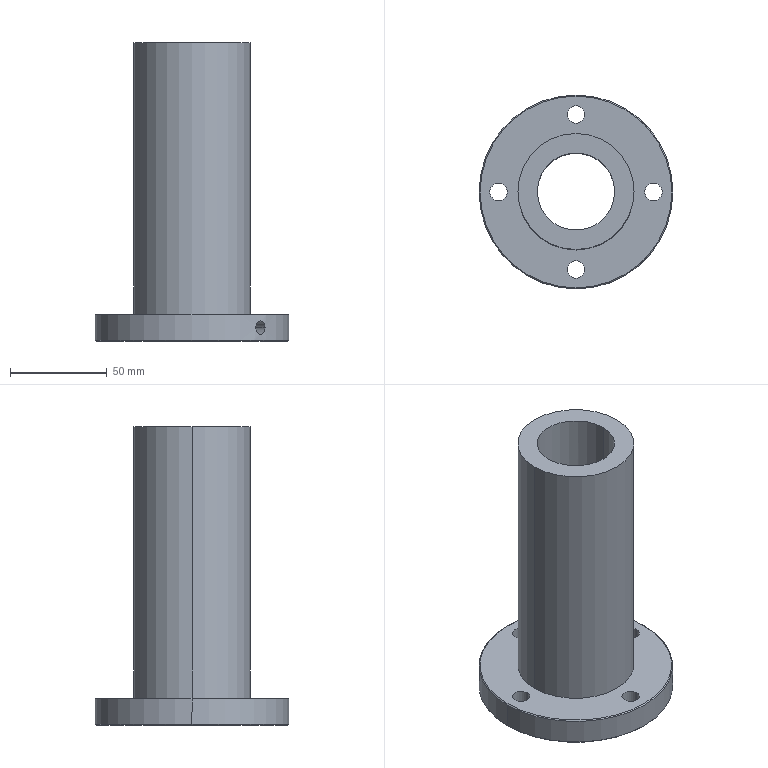Part | SolidWorks | features BaseBody 1 | 1 solid | 25 faces | box 100 x 100 x 154 mm | volume 306400 mm3 | cylinder 18 | cone 4 | plane 3 | commonest cylinder face diameters 9 x8 6.88 x4 40 x2 60 x2 100 x2
STEP:
#1=CARTESIAN_POINT('',(-30.,0.,147.));
#2=VERTEX_POINT('',#1);
#3=CARTESIAN_POINT('',(30.,0.,147.));
#4=VERTEX_POINT('',#3);
#5=CARTESIAN_POINT('',(0.,0.,147.));
#6=DIRECTION('',(0.,0.,-1.));
#7=DIRECTION('',(-1.,0.,0.));
#8=AXIS2_PLACEMENT_3D('',#5,#6,#7);
#9=CIRCLE('',#8,30.);
#10=EDGE_CURVE('',#2,#4,#9,.T.);
#11=ORIENTED_EDGE('',*,*,#10,.T.);
#12=CARTESIAN_POINT('',(30.,0.,7.));
#13=VERTEX_POINT('',#12);
#14=CARTESIAN_POINT('',(30.,0.,147.));
#15=DIRECTION('',(0.,0.,-1.));
#16=VECTOR('',#15,1000.);
#17=LINE('',#14,#16);
#18=EDGE_CURVE('',#4,#13,#17,.T.);
#19=ORIENTED_EDGE('',*,*,#18,.T.);
#20=CARTESIAN_POINT('',(-30.,0.,7.));
#21=VERTEX_POINT('',#20);
#22=CARTESIAN_POINT('',(0.,0.,7.));
#23=DIRECTION('',(0.,0.,1.));
#24=DIRECTION('',(-1.,0.,0.));
#25=AXIS2_PLACEMENT_3D('',#22,#23,#24);
#26=CIRCLE('',#25,30.);
#27=EDGE_CURVE('',#13,#21,#26,.T.);
#28=ORIENTED_EDGE('',*,*,#27,.T.);
#29=CARTESIAN_POINT('',(-30.,0.,147.));
#30=DIRECTION('',(0.,0.,-1.));
#31=VECTOR('',#30,1000.);
#32=LINE('',#29,#31);
#33=EDGE_CURVE('',#2,#21,#32,.T.);
#34=ORIENTED_EDGE('',*,*,#33,.F.);
#35=EDGE_LOOP('',(#11,#19,#28,#34));
#36=FACE_OUTER_BOUND('',#35,.T.);
#37=CARTESIAN_POINT('',(0.,0.,147.));
#38=DIRECTION('',(0.,0.,-1.));
#39=DIRECTION('',(-1.,0.,0.));
#40=AXIS2_PLACEMENT_3D('',#37,#38,#39);
#41=CYLINDRICAL_SURFACE('',#40,30.);
#42=ADVANCED_FACE('',(#36),#41,.T.);
#43=CARTESIAN_POINT('',(-4.5,-40.,-7.));
#44=VERTEX_POINT('',#43);
#45=CARTESIAN_POINT('',(4.5,-40.,-7.));
#46=VERTEX_POINT('',#45);
#47=CARTESIAN_POINT('',(0.,-40.,-7.));
#48=DIRECTION('',(0.,0.,1.));
#49=DIRECTION('',(1.,0.,0.));
#50=AXIS2_PLACEMENT_3D('',#47,#48,#49);
#51=CIRCLE('',#50,4.5);
#52=EDGE_CURVE('',#44,#46,#51,.T.);
#53=ORIENTED_EDGE('',*,*,#52,.F.);
#54=CARTESIAN_POINT('',(-4.5,-40.,7.));
#55=VERTEX_POINT('',#54);
#56=CARTESIAN_POINT('',(-4.5,-40.,-7.));
#57=DIRECTION('',(0.,0.,1.));
#58=VECTOR('',#57,1000.);
#59=LINE('',#56,#58);
#60=EDGE_CURVE('',#44,#55,#59,.T.);
#61=ORIENTED_EDGE('',*,*,#60,.T.);
#62=CARTESIAN_POINT('',(4.5,-40.,7.));
#63=VERTEX_POINT('',#62);
#64=CARTESIAN_POINT('',(0.,-40.,7.));
#65=DIRECTION('',(0.,0.,-1.));
#66=DIRECTION('',(1.,0.,0.));
#67=AXIS2_PLACEMENT_3D('',#64,#65,#66);
#68=CIRCLE('',#67,4.5);
#69=EDGE_CURVE('',#63,#55,#68,.T.);
#70=ORIENTED_EDGE('',*,*,#69,.F.);
#71=CARTESIAN_POINT('',(4.5,-40.,-7.));
#72=DIRECTION('',(0.,0.,1.));
#73=VECTOR('',#72,1000.);
#74=LINE('',#71,#73);
#75=EDGE_CURVE('',#46,#63,#74,.T.);
#76=ORIENTED_EDGE('',*,*,#75,.F.);
#77=EDGE_LOOP('',(#53,#61,#70,#76));
#78=FACE_OUTER_BOUND('',#77,.T.);
#79=CARTESIAN_POINT('',(0.,-40.,-7.));
#80=DIRECTION('',(0.,0.,1.));
#81=DIRECTION('',(1.,0.,0.));
#82=AXIS2_PLACEMENT_3D('',#79,#80,#81);
#83=CYLINDRICAL_SURFACE('',#82,4.5);
#84=ADVANCED_FACE('',(#78),#83,.F.);
#85=CARTESIAN_POINT('',(35.5,0.,-7.));
#86=VERTEX_POINT('',#85);
#87=CARTESIAN_POINT('',(44.5,0.,-7.));
#88=VERTEX_POINT('',#87);
#89=CARTESIAN_POINT('',(40.,0.,-7.));
#90=DIRECTION('',(0.,0.,1.));
#91=DIRECTION('',(1.,0.,0.));
#92=AXIS2_PLACEMENT_3D('',#89,#90,#91);
#93=CIRCLE('',#92,4.5);
#94=EDGE_CURVE('',#86,#88,#93,.T.);
#95=ORIENTED_EDGE('',*,*,#94,.F.);
#96=CARTESIAN_POINT('',(35.5,0.,7.));
#97=VERTEX_POINT('',#96);
#98=CARTESIAN_POINT('',(35.5,0.,-7.));
#99=DIRECTION('',(0.,0.,1.));
#100=VECTOR('',#99,1000.);
#101=LINE('',#98,#100);
#102=EDGE_CURVE('',#86,#97,#101,.T.);
#103=ORIENTED_EDGE('',*,*,#102,.T.);
#104=CARTESIAN_POINT('',(44.5,0.,7.));
#105=VERTEX_POINT('',#104);
#106=CARTESIAN_POINT('',(40.,0.,7.));
#107=DIRECTION('',(0.,0.,-1.));
#108=DIRECTION('',(1.,0.,0.));
#109=AXIS2_PLACEMENT_3D('',#106,#107,#108);
#110=CIRCLE('',#109,4.5);
#111=EDGE_CURVE('',#105,#97,#110,.T.);
#112=ORIENTED_EDGE('',*,*,#111,.F.);
#113=CARTESIAN_POINT('',(44.5,0.,-7.));
#114=DIRECTION('',(0.,0.,1.));
#115=VECTOR('',#114,1000.);
#116=LINE('',#113,#115);
#117=EDGE_CURVE('',#88,#105,#116,.T.);
#118=ORIENTED_EDGE('',*,*,#117,.F.);
#119=EDGE_LOOP('',(#95,#103,#112,#118));
#120=FACE_OUTER_BOUND('',#119,.T.);
#121=CARTESIAN_POINT('',(40.,0.,-7.));
#122=DIRECTION('',(0.,0.,1.));
#123=DIRECTION('',(1.,0.,0.));
#124=AXIS2_PLACEMENT_3D('',#121,#122,#123);
#125=CYLINDRICAL_SURFACE('',#124,4.5);
#126=ADVANCED_FACE('',(#120),#125,.F.);
#127=CARTESIAN_POINT('',(-4.5,40.,-7.));
#128=VERTEX_POINT('',#127);
#129=CARTESIAN_POINT('',(4.5,40.,-7.));
#130=VERTEX_POINT('',#129);
#131=CARTESIAN_POINT('',(0.,40.,-7.));
#132=DIRECTION('',(0.,0.,1.));
#133=DIRECTION('',(1.,0.,0.));
#134=AXIS2_PLACEMENT_3D('',#131,#132,#133);
#135=CIRCLE('',#134,4.5);
#136=EDGE_CURVE('',#128,#130,#135,.T.);
#137=ORIENTED_EDGE('',*,*,#136,.F.);
#138=CARTESIAN_POINT('',(-4.5,40.,7.));
#139=VERTEX_POINT('',#138);
#140=CARTESIAN_POINT('',(-4.5,40.,-7.));
#141=DIRECTION('',(0.,0.,1.));
#142=VECTOR('',#141,1000.);
#143=LINE('',#140,#142);
#144=EDGE_CURVE('',#128,#139,#143,.T.);
#145=ORIENTED_EDGE('',*,*,#144,.T.);
#146=CARTESIAN_POINT('',(4.5,40.,7.));
#147=VERTEX_POINT('',#146);
#148=CARTESIAN_POINT('',(0.,40.,7.));
#149=DIRECTION('',(0.,0.,-1.));
#150=DIRECTION('',(1.,0.,0.));
#151=AXIS2_PLACEMENT_3D('',#148,#149,#150);
#152=CIRCLE('',#151,4.5);
#153=EDGE_CURVE('',#147,#139,#152,.T.);
#154=ORIENTED_EDGE('',*,*,#153,.F.);
#155=CARTESIAN_POINT('',(4.5,40.,-7.));
#156=DIRECTION('',(0.,0.,1.));
#157=VECTOR('',#156,1000.);
#158=LINE('',#155,#157);
#159=EDGE_CURVE('',#130,#147,#158,.T.);
#160=ORIENTED_EDGE('',*,*,#159,.F.);
#161=EDGE_LOOP('',(#137,#145,#154,#160));
#162=FACE_OUTER_BOUND('',#161,.T.);
#163=CARTESIAN_POINT('',(0.,40.,-7.));
#164=DIRECTION('',(0.,0.,1.));
#165=DIRECTION('',(1.,0.,0.));
#166=AXIS2_PLACEMENT_3D('',#163,#164,#165);
#167=CYLINDRICAL_SURFACE('',#166,4.5);
#168=ADVANCED_FACE('',(#162),#167,.F.);
#169=CARTESIAN_POINT('',(-44.5,0.,-7.));
#170=VERTEX_POINT('',#169);
#171=CARTESIAN_POINT('',(-35.5,0.,-7.));
#172=VERTEX_POINT('',#171);
#173=CARTESIAN_POINT('',(-40.,0.,-7.));
#174=DIRECTION('',(0.,0.,1.));
#175=DIRECTION('',(1.,0.,0.));
#176=AXIS2_PLACEMENT_3D('',#173,#174,#175);
#177=CIRCLE('',#176,4.5);
#178=EDGE_CURVE('',#170,#172,#177,.T.);
#179=ORIENTED_EDGE('',*,*,#178,.F.);
#180=CARTESIAN_POINT('',(-44.5,0.,7.));
#181=VERTEX_POINT('',#180);
#182=CARTESIAN_POINT('',(-44.5,0.,-7.));
#183=DIRECTION('',(0.,0.,1.));
#184=VECTOR('',#183,1000.);
#185=LINE('',#182,#184);
#186=EDGE_CURVE('',#170,#181,#185,.T.);
#187=ORIENTED_EDGE('',*,*,#186,.T.);
#188=CARTESIAN_POINT('',(-35.5,0.,7.));
#189=VERTEX_POINT('',#188);
#190=CARTESIAN_POINT('',(-40.,0.,7.));
#191=DIRECTION('',(0.,0.,-1.));
#192=DIRECTION('',(1.,0.,0.));
#193=AXIS2_PLACEMENT_3D('',#190,#191,#192);
#194=CIRCLE('',#193,4.5);
#195=EDGE_CURVE('',#189,#181,#194,.T.);
#196=ORIENTED_EDGE('',*,*,#195,.F.);
#197=CARTESIAN_POINT('',(-35.5,0.,-7.));
#198=DIRECTION('',(0.,0.,1.));
#199=VECTOR('',#198,1000.);
#200=LINE('',#197,#199);
#201=EDGE_CURVE('',#172,#189,#200,.T.);
#202=ORIENTED_EDGE('',*,*,#201,.F.);
#203=EDGE_LOOP('',(#179,#187,#196,#202));
#204=FACE_OUTER_BOUND('',#203,.T.);
#205=CARTESIAN_POINT('',(-40.,0.,-7.));
#206=DIRECTION('',(0.,0.,1.));
#207=DIRECTION('',(1.,0.,0.));
#208=AXIS2_PLACEMENT_3D('',#205,#206,#207);
#209=CYLINDRICAL_SURFACE('',#208,4.5);
#210=ADVANCED_FACE('',(#204),#209,.F.);
#211=CARTESIAN_POINT('',(49.5,0.,7.));
#212=VERTEX_POINT('',#211);
#213=CARTESIAN_POINT('',(-49.5,0.,7.));
#214=VERTEX_POINT('',#213);
#215=CARTESIAN_POINT('',(0.,0.,7.));
#216=DIRECTION('',(0.,0.,1.));
#217=DIRECTION('',(-1.,0.,0.));
#218=AXIS2_PLACEMENT_3D('',#215,#216,#217);
#219=CIRCLE('',#218,49.5);
#220=EDGE_CURVE('',#212,#214,#219,.T.);
#221=ORIENTED_EDGE('',*,*,#220,.F.);
#222=CARTESIAN_POINT('',(50.,0.,6.5));
#223=VERTEX_POINT('',#222);
#224=CARTESIAN_POINT('',(50.,0.,6.5));
#225=DIRECTION('',(0.7071,0.,-0.7071));
#226=VECTOR('',#225,1000.);
#227=LINE('',#224,#226);
#228=EDGE_CURVE('',#212,#223,#227,.T.);
#229=ORIENTED_EDGE('',*,*,#228,.T.);
#230=CARTESIAN_POINT('',(-50.,0.,6.5));
#231=VERTEX_POINT('',#230);
#232=CARTESIAN_POINT('',(0.,0.,6.5));
#233=DIRECTION('',(0.,0.,1.));
#234=DIRECTION('',(-1.,0.,0.));
#235=AXIS2_PLACEMENT_3D('',#232,#233,#234);
#236=CIRCLE('',#235,50.);
#237=EDGE_CURVE('',#223,#231,#236,.T.);
#238=ORIENTED_EDGE('',*,*,#237,.T.);
#239=CARTESIAN_POINT('',(-50.,0.,6.5));
#240=DIRECTION('',(-0.7071,0.,-0.7071));
#241=VECTOR('',#240,1000.);
#242=LINE('',#239,#241);
#243=EDGE_CURVE('',#214,#231,#242,.T.);
#244=ORIENTED_EDGE('',*,*,#243,.F.);
#245=EDGE_LOOP('',(#221,#229,#238,#244));
#246=FACE_OUTER_BOUND('',#245,.T.);
#247=CARTESIAN_POINT('',(0.,0.,6.5));
#248=DIRECTION('',(0.,0.,-1.));
#249=DIRECTION('',(-1.,0.,0.));
#250=AXIS2_PLACEMENT_3D('',#247,#248,#249);
#251=CONICAL_SURFACE('',#250,50.,0.7854);
#252=ADVANCED_FACE('',(#246),#251,.T.);
#253=CARTESIAN_POINT('',(11.499,-16.364,0.));
#254=VERTEX_POINT('',#253);
#255=CARTESIAN_POINT('',(16.364,-11.499,0.));
#256=VERTEX_POINT('',#255);
#257=CARTESIAN_POINT('',(11.499,-16.364,0.));
#258=CARTESIAN_POINT('',(11.499,-16.364,0.2277));
#259=CARTESIAN_POINT('',(11.518,-16.351,0.4515));
#260=CARTESIAN_POINT('',(11.59,-16.299,0.8916));
#261=CARTESIAN_POINT('',(11.645,-16.26,1.11));
#262=CARTESIAN_POINT('',(11.787,-16.158,1.527));
#263=CARTESIAN_POINT('',(11.873,-16.095,1.724));
#264=CARTESIAN_POINT('',(12.075,-15.944,2.098));
#265=CARTESIAN_POINT('',(12.192,-15.855,2.274));
#266=CARTESIAN_POINT('',(12.443,-15.659,2.591));
#267=CARTESIAN_POINT('',(12.579,-15.55,2.733));
#268=CARTESIAN_POINT('',(12.87,-15.31,2.985));
#269=CARTESIAN_POINT('',(13.023,-15.181,3.091));
#270=CARTESIAN_POINT('',(13.335,-14.907,3.263));
#271=CARTESIAN_POINT('',(13.496,-14.762,3.329));
#272=CARTESIAN_POINT('',(13.821,-14.458,3.418));
#273=CARTESIAN_POINT('',(13.981,-14.303,3.44));
#274=CARTESIAN_POINT('',(14.299,-13.985,3.44));
#275=CARTESIAN_POINT('',(14.458,-13.821,3.418));
#276=CARTESIAN_POINT('',(14.76,-13.498,3.33));
#277=CARTESIAN_POINT('',(14.904,-13.339,3.265));
#278=CARTESIAN_POINT('',(15.179,-13.024,3.092));
#279=CARTESIAN_POINT('',(15.309,-12.871,2.985));
#280=CARTESIAN_POINT('',(15.547,-12.582,2.736));
#281=CARTESIAN_POINT('',(15.657,-12.445,2.594));
#282=CARTESIAN_POINT('',(15.856,-12.191,2.274));
#283=CARTESIAN_POINT('',(15.942,-12.077,2.101));
#284=CARTESIAN_POINT('',(16.093,-11.875,1.729));
#285=CARTESIAN_POINT('',(16.158,-11.787,1.527));
#286=CARTESIAN_POINT('',(16.26,-11.645,1.112));
#287=CARTESIAN_POINT('',(16.299,-11.591,0.8972));
#288=CARTESIAN_POINT('',(16.35,-11.518,0.4556));
#289=CARTESIAN_POINT('',(16.364,-11.499,0.2277));
#290=CARTESIAN_POINT('',(16.364,-11.499,0.));
#291=B_SPLINE_CURVE_WITH_KNOTS('',3,(#257,#258,#259,#260,#261,#262,#263,#264,#265,#266,#267,#268,#269,#270,#271,#272,#273,#274,#275,#276,#277,#278,#279,#280,#281,#282,#283,#284,#285,#286,#287,#288,#289,#290),.UNSPECIFIED.,.F.,.F.,(4,2,2,2,2,2,2,2,2,2,2,2,2,2,2,2,4),(0.,0.0006733,0.001347,0.00202,0.002693,0.003366,0.00404,0.004713,0.005386,0.006059,0.006733,0.007406,0.008079,0.008753,0.009426,0.0101,0.01077),.UNSPECIFIED.);
#292=EDGE_CURVE('',#254,#256,#291,.T.);
#293=ORIENTED_EDGE('',*,*,#292,.F.);
#294=CARTESIAN_POINT('',(16.364,-11.499,0.));
#295=CARTESIAN_POINT('',(16.364,-11.499,-0.2277));
#296=CARTESIAN_POINT('',(16.351,-11.518,-0.4515));
#297=CARTESIAN_POINT('',(16.299,-11.59,-0.8916));
#298=CARTESIAN_POINT('',(16.26,-11.645,-1.11));
#299=CARTESIAN_POINT('',(16.158,-11.787,-1.527));
#300=CARTESIAN_POINT('',(16.095,-11.873,-1.724));
#301=CARTESIAN_POINT('',(15.944,-12.075,-2.098));
#302=CARTESIAN_POINT('',(15.855,-12.192,-2.274));
#303=CARTESIAN_POINT('',(15.659,-12.443,-2.591));
#304=CARTESIAN_POINT('',(15.55,-12.579,-2.733));
#305=CARTESIAN_POINT('',(15.31,-12.87,-2.985));
#306=CARTESIAN_POINT('',(15.181,-13.023,-3.091));
#307=CARTESIAN_POINT('',(14.907,-13.335,-3.263));
#308=CARTESIAN_POINT('',(14.762,-13.496,-3.329));
#309=CARTESIAN_POINT('',(14.458,-13.821,-3.418));
#310=CARTESIAN_POINT('',(14.303,-13.981,-3.44));
#311=CARTESIAN_POINT('',(13.985,-14.299,-3.44));
#312=CARTESIAN_POINT('',(13.821,-14.458,-3.418));
#313=CARTESIAN_POINT('',(13.498,-14.76,-3.33));
#314=CARTESIAN_POINT('',(13.339,-14.904,-3.265));
#315=CARTESIAN_POINT('',(13.024,-15.179,-3.092));
#316=CARTESIAN_POINT('',(12.871,-15.309,-2.985));
#317=CARTESIAN_POINT('',(12.582,-15.547,-2.736));
#318=CARTESIAN_POINT('',(12.445,-15.657,-2.594));
#319=CARTESIAN_POINT('',(12.191,-15.856,-2.274));
#320=CARTESIAN_POINT('',(12.077,-15.942,-2.101));
#321=CARTESIAN_POINT('',(11.875,-16.093,-1.729));
#322=CARTESIAN_POINT('',(11.787,-16.158,-1.527));
#323=CARTESIAN_POINT('',(11.645,-16.26,-1.112));
#324=CARTESIAN_POINT('',(11.591,-16.299,-0.8972));
#325=CARTESIAN_POINT('',(11.518,-16.35,-0.4556));
#326=CARTESIAN_POINT('',(11.499,-16.364,-0.2277));
#327=CARTESIAN_POINT('',(11.499,-16.364,0.));
#328=B_SPLINE_CURVE_WITH_KNOTS('',3,(#294,#295,#296,#297,#298,#299,#300,#301,#302,#303,#304,#305,#306,#307,#308,#309,#310,#311,#312,#313,#314,#315,#316,#317,#318,#319,#320,#321,#322,#323,#324,#325,#326,#327),.UNSPECIFIED.,.F.,.F.,(4,2,2,2,2,2,2,2,2,2,2,2,2,2,2,2,4),(0.01077,0.01145,0.01212,0.01279,0.01347,0.01414,0.01481,0.01549,0.01616,0.01683,0.01751,0.01818,0.01885,0.01952,0.0202,0.02087,0.02154),.UNSPECIFIED.);
#329=EDGE_CURVE('',#256,#254,#328,.T.);
#330=ORIENTED_EDGE('',*,*,#329,.F.);
#331=EDGE_LOOP('',(#293,#330));
#332=FACE_BOUND('',#331,.T.);
#333=CARTESIAN_POINT('',(20.,0.,147.));
#334=VERTEX_POINT('',#333);
#335=CARTESIAN_POINT('',(-20.,0.,147.));
#336=VERTEX_POINT('',#335);
#337=CARTESIAN_POINT('',(0.,0.,147.));
#338=DIRECTION('',(0.,0.,-1.));
#339=DIRECTION('',(-1.,0.,0.));
#340=AXIS2_PLACEMENT_3D('',#337,#338,#339);
#341=CIRCLE('',#340,20.);
#342=EDGE_CURVE('',#334,#336,#341,.T.);
#343=ORIENTED_EDGE('',*,*,#342,.F.);
#344=CARTESIAN_POINT('',(20.,0.,-7.));
#345=VERTEX_POINT('',#344);
#346=CARTESIAN_POINT('',(20.,0.,7.));
#347=DIRECTION('',(0.,0.,-1.));
#348=VECTOR('',#347,1000.);
#349=LINE('',#346,#348);
#350=EDGE_CURVE('',#334,#345,#349,.T.);
#351=ORIENTED_EDGE('',*,*,#350,.T.);
#352=CARTESIAN_POINT('',(-20.,0.,-7.));
#353=VERTEX_POINT('',#352);
#354=CARTESIAN_POINT('',(0.,0.,-7.));
#355=DIRECTION('',(0.,0.,1.));
#356=DIRECTION('',(-1.,0.,0.));
#357=AXIS2_PLACEMENT_3D('',#354,#355,#356);
#358=CIRCLE('',#357,20.);
#359=EDGE_CURVE('',#353,#345,#358,.T.);
#360=ORIENTED_EDGE('',*,*,#359,.F.);
#361=CARTESIAN_POINT('',(-20.,0.,7.));
#362=DIRECTION('',(0.,0.,-1.));
#363=VECTOR('',#362,1000.);
#364=LINE('',#361,#363);
#365=EDGE_CURVE('',#336,#353,#364,.T.);
#366=ORIENTED_EDGE('',*,*,#365,.F.);
#367=EDGE_LOOP('',(#343,#351,#360,#366));
#368=FACE_OUTER_BOUND('',#367,.T.);
#369=CARTESIAN_POINT('',(0.,0.,7.));
#370=DIRECTION('',(0.,0.,-1.));
#371=DIRECTION('',(-1.,0.,0.));
#372=AXIS2_PLACEMENT_3D('',#369,#370,#371);
#373=CYLINDRICAL_SURFACE('',#372,20.);
#374=ADVANCED_FACE('',(#332,#368),#373,.F.);
#375=CARTESIAN_POINT('',(37.704,32.839,0.));
#376=VERTEX_POINT('',#375);
#377=CARTESIAN_POINT('',(32.839,37.704,0.));
#378=VERTEX_POINT('',#377);
#379=CARTESIAN_POINT('',(37.704,32.839,0.));
#380=CARTESIAN_POINT('',(37.704,32.839,0.2273));
#381=CARTESIAN_POINT('',(37.689,32.856,0.4508));
#382=CARTESIAN_POINT('',(37.632,32.922,0.8905));
#383=CARTESIAN_POINT('',(37.588,32.972,1.109));
#384=CARTESIAN_POINT('',(37.474,33.102,1.526));
#385=CARTESIAN_POINT('',(37.404,33.181,1.723));
#386=CARTESIAN_POINT('',(37.237,33.368,2.097));
#387=CARTESIAN_POINT('',(37.14,33.476,2.274));
#388=CARTESIAN_POINT('',(36.927,33.711,2.591));
#389=CARTESIAN_POINT('',(36.81,33.839,2.733));
#390=CARTESIAN_POINT('',(36.554,34.115,2.985));
#391=CARTESIAN_POINT('',(36.417,34.261,3.092));
#392=CARTESIAN_POINT('',(36.132,34.561,3.263));
#393=CARTESIAN_POINT('',(35.982,34.718,3.33));
#394=CARTESIAN_POINT('',(35.672,35.036,3.418));
#395=CARTESIAN_POINT('',(35.516,35.195,3.44));
#396=CARTESIAN_POINT('',(35.198,35.512,3.44));
#397=CARTESIAN_POINT('',(35.036,35.672,3.418));
#398=CARTESIAN_POINT('',(34.72,35.98,3.33));
#399=CARTESIAN_POINT('',(34.565,36.129,3.265));
#400=CARTESIAN_POINT('',(34.263,36.416,3.093));
#401=CARTESIAN_POINT('',(34.116,36.553,2.985));
#402=CARTESIAN_POINT('',(33.842,36.807,2.737));
#403=CARTESIAN_POINT('',(33.714,36.924,2.595));
#404=CARTESIAN_POINT('',(33.476,37.14,2.274));
#405=CARTESIAN_POINT('',(33.369,37.236,2.1));
#406=CARTESIAN_POINT('',(33.183,37.402,1.728));
#407=CARTESIAN_POINT('',(33.102,37.473,1.527));
#408=CARTESIAN_POINT('',(32.972,37.588,1.11));
#409=CARTESIAN_POINT('',(32.923,37.631,0.8956));
#410=CARTESIAN_POINT('',(32.856,37.689,0.4548));
#411=CARTESIAN_POINT('',(32.839,37.704,0.2273));
#412=CARTESIAN_POINT('',(32.839,37.704,0.));
#413=B_SPLINE_CURVE_WITH_KNOTS('',3,(#379,#380,#381,#382,#383,#384,#385,#386,#387,#388,#389,#390,#391,#392,#393,#394,#395,#396,#397,#398,#399,#400,#401,#402,#403,#404,#405,#406,#407,#408,#409,#410,#411,#412),.UNSPECIFIED.,.F.,.F.,(4,2,2,2,2,2,2,2,2,2,2,2,2,2,2,2,4),(0.,0.0006722,0.001344,0.002017,0.002689,0.003361,0.004033,0.004706,0.005378,0.00605,0.006722,0.007395,0.008067,0.008739,0.009411,0.01008,0.01076),.UNSPECIFIED.);
#414=EDGE_CURVE('',#376,#378,#413,.T.);
#415=ORIENTED_EDGE('',*,*,#414,.T.);
#416=CARTESIAN_POINT('',(32.839,37.704,0.));
#417=CARTESIAN_POINT('',(32.839,37.704,-0.2273));
#418=CARTESIAN_POINT('',(32.856,37.689,-0.4508));
#419=CARTESIAN_POINT('',(32.922,37.632,-0.8905));
#420=CARTESIAN_POINT('',(32.972,37.588,-1.109));
#421=CARTESIAN_POINT('',(33.102,37.474,-1.526));
#422=CARTESIAN_POINT('',(33.181,37.404,-1.723));
#423=CARTESIAN_POINT('',(33.368,37.237,-2.097));
#424=CARTESIAN_POINT('',(33.476,37.14,-2.274));
#425=CARTESIAN_POINT('',(33.711,36.927,-2.591));
#426=CARTESIAN_POINT('',(33.839,36.81,-2.733));
#427=CARTESIAN_POINT('',(34.115,36.554,-2.985));
#428=CARTESIAN_POINT('',(34.261,36.417,-3.092));
#429=CARTESIAN_POINT('',(34.561,36.132,-3.263));
#430=CARTESIAN_POINT('',(34.718,35.982,-3.33));
#431=CARTESIAN_POINT('',(35.036,35.672,-3.418));
#432=CARTESIAN_POINT('',(35.195,35.516,-3.44));
#433=CARTESIAN_POINT('',(35.512,35.198,-3.44));
#434=CARTESIAN_POINT('',(35.672,35.036,-3.418));
#435=CARTESIAN_POINT('',(35.98,34.72,-3.33));
#436=CARTESIAN_POINT('',(36.129,34.565,-3.265));
#437=CARTESIAN_POINT('',(36.416,34.263,-3.093));
#438=CARTESIAN_POINT('',(36.553,34.116,-2.985));
#439=CARTESIAN_POINT('',(36.807,33.842,-2.737));
#440=CARTESIAN_POINT('',(36.924,33.714,-2.595));
#441=CARTESIAN_POINT('',(37.14,33.476,-2.274));
#442=CARTESIAN_POINT('',(37.236,33.369,-2.1));
#443=CARTESIAN_POINT('',(37.402,33.183,-1.728));
#444=CARTESIAN_POINT('',(37.473,33.102,-1.527));
#445=CARTESIAN_POINT('',(37.588,32.972,-1.11));
#446=CARTESIAN_POINT('',(37.631,32.923,-0.8956));
#447=CARTESIAN_POINT('',(37.689,32.856,-0.4548));
#448=CARTESIAN_POINT('',(37.704,32.839,-0.2273));
#449=CARTESIAN_POINT('',(37.704,32.839,0.));
#450=B_SPLINE_CURVE_WITH_KNOTS('',3,(#416,#417,#418,#419,#420,#421,#422,#423,#424,#425,#426,#427,#428,#429,#430,#431,#432,#433,#434,#435,#436,#437,#438,#439,#440,#441,#442,#443,#444,#445,#446,#447,#448,#449),.UNSPECIFIED.,.F.,.F.,(4,2,2,2,2,2,2,2,2,2,2,2,2,2,2,2,4),(0.01076,0.01143,0.0121,0.01277,0.01344,0.01412,0.01479,0.01546,0.01613,0.01681,0.01748,0.01815,0.01882,0.0195,0.02017,0.02084,0.02151),.UNSPECIFIED.);
#451=EDGE_CURVE('',#378,#376,#450,.T.);
#452=ORIENTED_EDGE('',*,*,#451,.T.);
#453=EDGE_LOOP('',(#415,#452));
#454=FACE_BOUND('',#453,.T.);
#455=ORIENTED_EDGE('',*,*,#237,.F.);
#456=CARTESIAN_POINT('',(50.,0.,-6.5));
#457=VERTEX_POINT('',#456);
#458=CARTESIAN_POINT('',(50.,0.,7.));
#459=DIRECTION('',(0.,0.,-1.));
#460=VECTOR('',#459,1000.);
#461=LINE('',#458,#460);
#462=EDGE_CURVE('',#223,#457,#461,.T.);
#463=ORIENTED_EDGE('',*,*,#462,.T.);
#464=CARTESIAN_POINT('',(-50.,0.,-6.5));
#465=VERTEX_POINT('',#464);
#466=CARTESIAN_POINT('',(0.,0.,-6.5));
#467=DIRECTION('',(0.,0.,1.));
#468=DIRECTION('',(-1.,0.,0.));
#469=AXIS2_PLACEMENT_3D('',#466,#467,#468);
#470=CIRCLE('',#469,50.);
#471=EDGE_CURVE('',#457,#465,#470,.T.);
#472=ORIENTED_EDGE('',*,*,#471,.T.);
#473=CARTESIAN_POINT('',(-50.,0.,7.));
#474=DIRECTION('',(0.,0.,-1.));
#475=VECTOR('',#474,1000.);
#476=LINE('',#473,#475);
#477=EDGE_CURVE('',#231,#465,#476,.T.);
#478=ORIENTED_EDGE('',*,*,#477,.F.);
#479=EDGE_LOOP('',(#455,#463,#472,#478));
#480=FACE_OUTER_BOUND('',#479,.T.);
#481=CARTESIAN_POINT('',(0.,0.,7.));
#482=DIRECTION('',(0.,0.,-1.));
#483=DIRECTION('',(-1.,0.,0.));
#484=AXIS2_PLACEMENT_3D('',#481,#482,#483);
#485=CYLINDRICAL_SURFACE('',#484,50.);
#486=ADVANCED_FACE('',(#454,#480),#485,.T.);
#487=ORIENTED_EDGE('',*,*,#451,.F.);
#488=CARTESIAN_POINT('',(11.499,16.364,0.));
#489=VERTEX_POINT('',#488);
#490=CARTESIAN_POINT('',(47.568,52.432,0.));
#491=DIRECTION('',(-0.7071,-0.7071,0.));
#492=VECTOR('',#491,1000.);
#493=LINE('',#490,#492);
#494=EDGE_CURVE('',#378,#489,#493,.T.);
#495=ORIENTED_EDGE('',*,*,#494,.T.);
#496=CARTESIAN_POINT('',(16.364,11.499,0.));
#497=VERTEX_POINT('',#496);
#498=CARTESIAN_POINT('',(11.499,16.364,0.));
#499=CARTESIAN_POINT('',(11.499,16.364,-0.2277));
#500=CARTESIAN_POINT('',(11.518,16.351,-0.4515));
#501=CARTESIAN_POINT('',(11.59,16.299,-0.8916));
#502=CARTESIAN_POINT('',(11.645,16.26,-1.11));
#503=CARTESIAN_POINT('',(11.787,16.158,-1.527));
#504=CARTESIAN_POINT('',(11.873,16.095,-1.724));
#505=CARTESIAN_POINT('',(12.075,15.944,-2.098));
#506=CARTESIAN_POINT('',(12.192,15.855,-2.274));
#507=CARTESIAN_POINT('',(12.443,15.659,-2.591));
#508=CARTESIAN_POINT('',(12.579,15.55,-2.733));
#509=CARTESIAN_POINT('',(12.87,15.31,-2.985));
#510=CARTESIAN_POINT('',(13.023,15.181,-3.091));
#511=CARTESIAN_POINT('',(13.335,14.907,-3.263));
#512=CARTESIAN_POINT('',(13.496,14.762,-3.329));
#513=CARTESIAN_POINT('',(13.821,14.458,-3.418));
#514=CARTESIAN_POINT('',(13.981,14.303,-3.44));
#515=CARTESIAN_POINT('',(14.299,13.985,-3.44));
#516=CARTESIAN_POINT('',(14.458,13.821,-3.418));
#517=CARTESIAN_POINT('',(14.76,13.498,-3.33));
#518=CARTESIAN_POINT('',(14.904,13.339,-3.265));
#519=CARTESIAN_POINT('',(15.179,13.024,-3.092));
#520=CARTESIAN_POINT('',(15.309,12.871,-2.985));
#521=CARTESIAN_POINT('',(15.547,12.582,-2.736));
#522=CARTESIAN_POINT('',(15.657,12.445,-2.594));
#523=CARTESIAN_POINT('',(15.856,12.191,-2.274));
#524=CARTESIAN_POINT('',(15.942,12.077,-2.101));
#525=CARTESIAN_POINT('',(16.093,11.875,-1.729));
#526=CARTESIAN_POINT('',(16.158,11.787,-1.527));
#527=CARTESIAN_POINT('',(16.26,11.645,-1.112));
#528=CARTESIAN_POINT('',(16.299,11.591,-0.8972));
#529=CARTESIAN_POINT('',(16.35,11.518,-0.4556));
#530=CARTESIAN_POINT('',(16.364,11.499,-0.2277));
#531=CARTESIAN_POINT('',(16.364,11.499,0.));
#532=B_SPLINE_CURVE_WITH_KNOTS('',3,(#498,#499,#500,#501,#502,#503,#504,#505,#506,#507,#508,#509,#510,#511,#512,#513,#514,#515,#516,#517,#518,#519,#520,#521,#522,#523,#524,#525,#526,#527,#528,#529,#530,#531),.UNSPECIFIED.,.F.,.F.,(4,2,2,2,2,2,2,2,2,2,2,2,2,2,2,2,4),(0.,0.0006733,0.001347,0.00202,0.002693,0.003366,0.00404,0.004713,0.005386,0.006059,0.006733,0.007406,0.008079,0.008753,0.009426,0.0101,0.01077),.UNSPECIFIED.);
#533=EDGE_CURVE('',#489,#497,#532,.T.);
#534=ORIENTED_EDGE('',*,*,#533,.T.);
#535=CARTESIAN_POINT('',(52.432,47.568,0.));
#536=DIRECTION('',(-0.7071,-0.7071,0.));
#537=VECTOR('',#536,1000.);
#538=LINE('',#535,#537);
#539=EDGE_CURVE('',#376,#497,#538,.T.);
#540=ORIENTED_EDGE('',*,*,#539,.F.);
#541=EDGE_LOOP('',(#487,#495,#534,#540));
#542=FACE_OUTER_BOUND('',#541,.T.);
#543=CARTESIAN_POINT('',(50.,50.,0.));
#544=DIRECTION('',(-0.7071,-0.7071,0.));
#545=DIRECTION('',(0.7071,-0.7071,0.));
#546=AXIS2_PLACEMENT_3D('',#543,#544,#545);
#547=CYLINDRICAL_SURFACE('',#546,3.44);
#548=ADVANCED_FACE('',(#542),#547,.F.);
#549=CARTESIAN_POINT('',(37.704,-32.839,0.));
#550=VERTEX_POINT('',#549);
#551=CARTESIAN_POINT('',(32.839,-37.704,0.));
#552=VERTEX_POINT('',#551);
#553=CARTESIAN_POINT('',(37.704,-32.839,0.));
#554=CARTESIAN_POINT('',(37.704,-32.839,-0.2273));
#555=CARTESIAN_POINT('',(37.689,-32.856,-0.4508));
#556=CARTESIAN_POINT('',(37.632,-32.922,-0.8905));
#557=CARTESIAN_POINT('',(37.588,-32.972,-1.109));
#558=CARTESIAN_POINT('',(37.474,-33.102,-1.526));
#559=CARTESIAN_POINT('',(37.404,-33.181,-1.723));
#560=CARTESIAN_POINT('',(37.237,-33.368,-2.097));
#561=CARTESIAN_POINT('',(37.14,-33.476,-2.274));
#562=CARTESIAN_POINT('',(36.927,-33.711,-2.591));
#563=CARTESIAN_POINT('',(36.81,-33.839,-2.733));
#564=CARTESIAN_POINT('',(36.554,-34.115,-2.985));
#565=CARTESIAN_POINT('',(36.417,-34.261,-3.092));
#566=CARTESIAN_POINT('',(36.132,-34.561,-3.263));
#567=CARTESIAN_POINT('',(35.982,-34.718,-3.33));
#568=CARTESIAN_POINT('',(35.672,-35.036,-3.418));
#569=CARTESIAN_POINT('',(35.516,-35.195,-3.44));
#570=CARTESIAN_POINT('',(35.198,-35.512,-3.44));
#571=CARTESIAN_POINT('',(35.036,-35.672,-3.418));
#572=CARTESIAN_POINT('',(34.72,-35.98,-3.33));
#573=CARTESIAN_POINT('',(34.565,-36.129,-3.265));
#574=CARTESIAN_POINT('',(34.263,-36.416,-3.093));
#575=CARTESIAN_POINT('',(34.116,-36.553,-2.985));
#576=CARTESIAN_POINT('',(33.842,-36.807,-2.737));
#577=CARTESIAN_POINT('',(33.714,-36.924,-2.595));
#578=CARTESIAN_POINT('',(33.476,-37.14,-2.274));
#579=CARTESIAN_POINT('',(33.369,-37.236,-2.1));
#580=CARTESIAN_POINT('',(33.183,-37.402,-1.728));
#581=CARTESIAN_POINT('',(33.102,-37.473,-1.527));
#582=CARTESIAN_POINT('',(32.972,-37.588,-1.11));
#583=CARTESIAN_POINT('',(32.923,-37.631,-0.8956));
#584=CARTESIAN_POINT('',(32.856,-37.689,-0.4548));
#585=CARTESIAN_POINT('',(32.839,-37.704,-0.2273));
#586=CARTESIAN_POINT('',(32.839,-37.704,0.));
#587=B_SPLINE_CURVE_WITH_KNOTS('',3,(#553,#554,#555,#556,#557,#558,#559,#560,#561,#562,#563,#564,#565,#566,#567,#568,#569,#570,#571,#572,#573,#574,#575,#576,#577,#578,#579,#580,#581,#582,#583,#584,#585,#586),.UNSPECIFIED.,.F.,.F.,(4,2,2,2,2,2,2,2,2,2,2,2,2,2,2,2,4),(0.,0.0006722,0.001344,0.002017,0.002689,0.003361,0.004033,0.004706,0.005378,0.00605,0.006722,0.007395,0.008067,0.008739,0.009411,0.01008,0.01076),.UNSPECIFIED.);
#588=EDGE_CURVE('',#550,#552,#587,.T.);
#589=ORIENTED_EDGE('',*,*,#588,.F.);
#590=CARTESIAN_POINT('',(52.432,-47.568,0.));
#591=DIRECTION('',(-0.7071,0.7071,0.));
#592=VECTOR('',#591,1000.);
#593=LINE('',#590,#592);
#594=EDGE_CURVE('',#550,#256,#593,.T.);
#595=ORIENTED_EDGE('',*,*,#594,.T.);
#596=ORIENTED_EDGE('',*,*,#329,.T.);
#597=CARTESIAN_POINT('',(47.568,-52.432,0.));
#598=DIRECTION('',(-0.7071,0.7071,0.));
#599=VECTOR('',#598,1000.);
#600=LINE('',#597,#599);
#601=EDGE_CURVE('',#552,#254,#600,.T.);
#602=ORIENTED_EDGE('',*,*,#601,.F.);
#603=EDGE_LOOP('',(#589,#595,#596,#602));
#604=FACE_OUTER_BOUND('',#603,.T.);
#605=CARTESIAN_POINT('',(50.,-50.,0.));
#606=DIRECTION('',(-0.7071,0.7071,0.));
#607=DIRECTION('',(-0.7071,-0.7071,0.));
#608=AXIS2_PLACEMENT_3D('',#605,#606,#607);
#609=CYLINDRICAL_SURFACE('',#608,3.44);
#610=ADVANCED_FACE('',(#604),#609,.F.);
#611=CARTESIAN_POINT('',(49.5,0.,-7.));
#612=VERTEX_POINT('',#611);
#613=CARTESIAN_POINT('',(-49.5,0.,-7.));
#614=VERTEX_POINT('',#613);
#615=CARTESIAN_POINT('',(0.,0.,-7.));
#616=DIRECTION('',(0.,0.,1.));
#617=DIRECTION('',(1.,0.,0.));
#618=AXIS2_PLACEMENT_3D('',#615,#616,#617);
#619=CIRCLE('',#618,49.5);
#620=EDGE_CURVE('',#612,#614,#619,.T.);
#621=ORIENTED_EDGE('',*,*,#620,.T.);
#622=CARTESIAN_POINT('',(-50.,0.,-6.5));
#623=DIRECTION('',(-0.7071,0.,0.7071));
#624=VECTOR('',#623,1000.);
#625=LINE('',#622,#624);
#626=EDGE_CURVE('',#614,#465,#625,.T.);
#627=ORIENTED_EDGE('',*,*,#626,.T.);
#628=ORIENTED_EDGE('',*,*,#471,.F.);
#629=CARTESIAN_POINT('',(50.,0.,-6.5));
#630=DIRECTION('',(0.7071,0.,0.7071));
#631=VECTOR('',#630,1000.);
#632=LINE('',#629,#631);
#633=EDGE_CURVE('',#612,#457,#632,.T.);
#634=ORIENTED_EDGE('',*,*,#633,.F.);
#635=EDGE_LOOP('',(#621,#627,#628,#634));
#636=FACE_OUTER_BOUND('',#635,.T.);
#637=CARTESIAN_POINT('',(0.,0.,-6.5));
#638=DIRECTION('',(0.,0.,1.));
#639=DIRECTION('',(1.,0.,0.));
#640=AXIS2_PLACEMENT_3D('',#637,#638,#639);
#641=CONICAL_SURFACE('',#640,50.,0.7854);
#642=ADVANCED_FACE('',(#636),#641,.T.);
#643=ORIENTED_EDGE('',*,*,#18,.F.);
#644=CARTESIAN_POINT('',(0.,0.,147.));
#645=DIRECTION('',(0.,0.,-1.));
#646=DIRECTION('',(-1.,0.,0.));
#647=AXIS2_PLACEMENT_3D('',#644,#645,#646);
#648=CIRCLE('',#647,30.);
#649=EDGE_CURVE('',#4,#2,#648,.T.);
#650=ORIENTED_EDGE('',*,*,#649,.T.);
#651=ORIENTED_EDGE('',*,*,#33,.T.);
#652=CARTESIAN_POINT('',(0.,0.,7.));
#653=DIRECTION('',(0.,0.,1.));
#654=DIRECTION('',(-1.,0.,0.));
#655=AXIS2_PLACEMENT_3D('',#652,#653,#654);
#656=CIRCLE('',#655,30.);
#657=EDGE_CURVE('',#21,#13,#656,.T.);
#658=ORIENTED_EDGE('',*,*,#657,.T.);
#659=EDGE_LOOP('',(#643,#650,#651,#658));
#660=FACE_OUTER_BOUND('',#659,.T.);
#661=CARTESIAN_POINT('',(0.,0.,147.));
#662=DIRECTION('',(0.,0.,-1.));
#663=DIRECTION('',(-1.,0.,0.));
#664=AXIS2_PLACEMENT_3D('',#661,#662,#663);
#665=CYLINDRICAL_SURFACE('',#664,30.);
#666=ADVANCED_FACE('',(#660),#665,.T.);
#667=ORIENTED_EDGE('',*,*,#657,.F.);
#668=ORIENTED_EDGE('',*,*,#27,.F.);
#669=EDGE_LOOP('',(#667,#668));
#670=FACE_BOUND('',#669,.T.);
#671=ORIENTED_EDGE('',*,*,#69,.T.);
#672=CARTESIAN_POINT('',(0.,-40.,7.));
#673=DIRECTION('',(0.,0.,-1.));
#674=DIRECTION('',(1.,0.,0.));
#675=AXIS2_PLACEMENT_3D('',#672,#673,#674);
#676=CIRCLE('',#675,4.5);
#677=EDGE_CURVE('',#55,#63,#676,.T.);
#678=ORIENTED_EDGE('',*,*,#677,.T.);
#679=EDGE_LOOP('',(#671,#678));
#680=FACE_BOUND('',#679,.T.);
#681=ORIENTED_EDGE('',*,*,#111,.T.);
#682=CARTESIAN_POINT('',(40.,0.,7.));
#683=DIRECTION('',(0.,0.,-1.));
#684=DIRECTION('',(1.,0.,0.));
#685=AXIS2_PLACEMENT_3D('',#682,#683,#684);
#686=CIRCLE('',#685,4.5);
#687=EDGE_CURVE('',#97,#105,#686,.T.);
#688=ORIENTED_EDGE('',*,*,#687,.T.);
#689=EDGE_LOOP('',(#681,#688));
#690=FACE_BOUND('',#689,.T.);
#691=ORIENTED_EDGE('',*,*,#153,.T.);
#692=CARTESIAN_POINT('',(0.,40.,7.));
#693=DIRECTION('',(0.,0.,-1.));
#694=DIRECTION('',(1.,0.,0.));
#695=AXIS2_PLACEMENT_3D('',#692,#693,#694);
#696=CIRCLE('',#695,4.5);
#697=EDGE_CURVE('',#139,#147,#696,.T.);
#698=ORIENTED_EDGE('',*,*,#697,.T.);
#699=EDGE_LOOP('',(#691,#698));
#700=FACE_BOUND('',#699,.T.);
#701=ORIENTED_EDGE('',*,*,#195,.T.);
#702=CARTESIAN_POINT('',(-40.,0.,7.));
#703=DIRECTION('',(0.,0.,-1.));
#704=DIRECTION('',(1.,0.,0.));
#705=AXIS2_PLACEMENT_3D('',#702,#703,#704);
#706=CIRCLE('',#705,4.5);
#707=EDGE_CURVE('',#181,#189,#706,.T.);
#708=ORIENTED_EDGE('',*,*,#707,.T.);
#709=EDGE_LOOP('',(#701,#708));
#710=FACE_BOUND('',#709,.T.);
#711=CARTESIAN_POINT('',(0.,0.,7.));
#712=DIRECTION('',(0.,0.,1.));
#713=DIRECTION('',(-1.,0.,0.));
#714=AXIS2_PLACEMENT_3D('',#711,#712,#713);
#715=CIRCLE('',#714,49.5);
#716=EDGE_CURVE('',#214,#212,#715,.T.);
#717=ORIENTED_EDGE('',*,*,#716,.T.);
#718=ORIENTED_EDGE('',*,*,#220,.T.);
#719=EDGE_LOOP('',(#717,#718));
#720=FACE_OUTER_BOUND('',#719,.T.);
#721=CARTESIAN_POINT('',(0.,0.,7.));
#722=DIRECTION('',(0.,0.,1.));
#723=DIRECTION('',(1.,0.,0.));
#724=AXIS2_PLACEMENT_3D('',#721,#722,#723);
#725=PLANE('',#724);
#726=ADVANCED_FACE('',(#670,#680,#690,#700,#710,#720),#725,.T.);
#727=CARTESIAN_POINT('',(0.,0.,147.));
#728=DIRECTION('',(0.,0.,-1.));
#729=DIRECTION('',(-1.,0.,0.));
#730=AXIS2_PLACEMENT_3D('',#727,#728,#729);
#731=CIRCLE('',#730,20.);
#732=EDGE_CURVE('',#336,#334,#731,.T.);
#733=ORIENTED_EDGE('',*,*,#732,.T.);
#734=ORIENTED_EDGE('',*,*,#342,.T.);
#735=EDGE_LOOP('',(#733,#734));
#736=FACE_BOUND('',#735,.T.);
#737=ORIENTED_EDGE('',*,*,#10,.F.);
#738=ORIENTED_EDGE('',*,*,#649,.F.);
#739=EDGE_LOOP('',(#737,#738));
#740=FACE_OUTER_BOUND('',#739,.T.);
#741=CARTESIAN_POINT('',(0.,0.,147.));
#742=DIRECTION('',(0.,0.,1.));
#743=DIRECTION('',(1.,0.,0.));
#744=AXIS2_PLACEMENT_3D('',#741,#742,#743);
#745=PLANE('',#744);
#746=ADVANCED_FACE('',(#736,#740),#745,.T.);
#747=ORIENTED_EDGE('',*,*,#60,.F.);
#748=CARTESIAN_POINT('',(0.,-40.,-7.));
#749=DIRECTION('',(0.,0.,1.));
#750=DIRECTION('',(1.,0.,0.));
#751=AXIS2_PLACEMENT_3D('',#748,#749,#750);
#752=CIRCLE('',#751,4.5);
#753=EDGE_CURVE('',#46,#44,#752,.T.);
#754=ORIENTED_EDGE('',*,*,#753,.F.);
#755=ORIENTED_EDGE('',*,*,#75,.T.);
#756=ORIENTED_EDGE('',*,*,#677,.F.);
#757=EDGE_LOOP('',(#747,#754,#755,#756));
#758=FACE_OUTER_BOUND('',#757,.T.);
#759=CARTESIAN_POINT('',(0.,-40.,-7.));
#760=DIRECTION('',(0.,0.,1.));
#761=DIRECTION('',(1.,0.,0.));
#762=AXIS2_PLACEMENT_3D('',#759,#760,#761);
#763=CYLINDRICAL_SURFACE('',#762,4.5);
#764=ADVANCED_FACE('',(#758),#763,.F.);
#765=ORIENTED_EDGE('',*,*,#102,.F.);
#766=CARTESIAN_POINT('',(40.,0.,-7.));
#767=DIRECTION('',(0.,0.,1.));
#768=DIRECTION('',(1.,0.,0.));
#769=AXIS2_PLACEMENT_3D('',#766,#767,#768);
#770=CIRCLE('',#769,4.5);
#771=EDGE_CURVE('',#88,#86,#770,.T.);
#772=ORIENTED_EDGE('',*,*,#771,.F.);
#773=ORIENTED_EDGE('',*,*,#117,.T.);
#774=ORIENTED_EDGE('',*,*,#687,.F.);
#775=EDGE_LOOP('',(#765,#772,#773,#774));
#776=FACE_OUTER_BOUND('',#775,.T.);
#777=CARTESIAN_POINT('',(40.,0.,-7.));
#778=DIRECTION('',(0.,0.,1.));
#779=DIRECTION('',(1.,0.,0.));
#780=AXIS2_PLACEMENT_3D('',#777,#778,#779);
#781=CYLINDRICAL_SURFACE('',#780,4.5);
#782=ADVANCED_FACE('',(#776),#781,.F.);
#783=ORIENTED_EDGE('',*,*,#144,.F.);
#784=CARTESIAN_POINT('',(0.,40.,-7.));
#785=DIRECTION('',(0.,0.,1.));
#786=DIRECTION('',(1.,0.,0.));
#787=AXIS2_PLACEMENT_3D('',#784,#785,#786);
#788=CIRCLE('',#787,4.5);
#789=EDGE_CURVE('',#130,#128,#788,.T.);
#790=ORIENTED_EDGE('',*,*,#789,.F.);
#791=ORIENTED_EDGE('',*,*,#159,.T.);
#792=ORIENTED_EDGE('',*,*,#697,.F.);
#793=EDGE_LOOP('',(#783,#790,#791,#792));
#794=FACE_OUTER_BOUND('',#793,.T.);
#795=CARTESIAN_POINT('',(0.,40.,-7.));
#796=DIRECTION('',(0.,0.,1.));
#797=DIRECTION('',(1.,0.,0.));
#798=AXIS2_PLACEMENT_3D('',#795,#796,#797);
#799=CYLINDRICAL_SURFACE('',#798,4.5);
#800=ADVANCED_FACE('',(#794),#799,.F.);
#801=ORIENTED_EDGE('',*,*,#186,.F.);
#802=CARTESIAN_POINT('',(-40.,0.,-7.));
#803=DIRECTION('',(0.,0.,1.));
#804=DIRECTION('',(1.,0.,0.));
#805=AXIS2_PLACEMENT_3D('',#802,#803,#804);
#806=CIRCLE('',#805,4.5);
#807=EDGE_CURVE('',#172,#170,#806,.T.);
#808=ORIENTED_EDGE('',*,*,#807,.F.);
#809=ORIENTED_EDGE('',*,*,#201,.T.);
#810=ORIENTED_EDGE('',*,*,#707,.F.);
#811=EDGE_LOOP('',(#801,#808,#809,#810));
#812=FACE_OUTER_BOUND('',#811,.T.);
#813=CARTESIAN_POINT('',(-40.,0.,-7.));
#814=DIRECTION('',(0.,0.,1.));
#815=DIRECTION('',(1.,0.,0.));
#816=AXIS2_PLACEMENT_3D('',#813,#814,#815);
#817=CYLINDRICAL_SURFACE('',#816,4.5);
#818=ADVANCED_FACE('',(#812),#817,.F.);
#819=ORIENTED_EDGE('',*,*,#228,.F.);
#820=ORIENTED_EDGE('',*,*,#716,.F.);
#821=ORIENTED_EDGE('',*,*,#243,.T.);
#822=CARTESIAN_POINT('',(0.,0.,6.5));
#823=DIRECTION('',(0.,0.,1.));
#824=DIRECTION('',(-1.,0.,0.));
#825=AXIS2_PLACEMENT_3D('',#822,#823,#824);
#826=CIRCLE('',#825,50.);
#827=EDGE_CURVE('',#231,#223,#826,.T.);
#828=ORIENTED_EDGE('',*,*,#827,.T.);
#829=EDGE_LOOP('',(#819,#820,#821,#828));
#830=FACE_OUTER_BOUND('',#829,.T.);
#831=CARTESIAN_POINT('',(0.,0.,6.5));
#832=DIRECTION('',(0.,0.,-1.));
#833=DIRECTION('',(-1.,0.,0.));
#834=AXIS2_PLACEMENT_3D('',#831,#832,#833);
#835=CONICAL_SURFACE('',#834,50.,0.7854);
#836=ADVANCED_FACE('',(#830),#835,.T.);
#837=ORIENTED_EDGE('',*,*,#350,.F.);
#838=ORIENTED_EDGE('',*,*,#732,.F.);
#839=ORIENTED_EDGE('',*,*,#365,.T.);
#840=CARTESIAN_POINT('',(0.,0.,-7.));
#841=DIRECTION('',(0.,0.,1.));
#842=DIRECTION('',(-1.,0.,0.));
#843=AXIS2_PLACEMENT_3D('',#840,#841,#842);
#844=CIRCLE('',#843,20.);
#845=EDGE_CURVE('',#345,#353,#844,.T.);
#846=ORIENTED_EDGE('',*,*,#845,.F.);
#847=EDGE_LOOP('',(#837,#838,#839,#846));
#848=FACE_OUTER_BOUND('',#847,.T.);
#849=CARTESIAN_POINT('',(16.364,11.499,0.));
#850=CARTESIAN_POINT('',(16.364,11.499,0.2277));
#851=CARTESIAN_POINT('',(16.351,11.518,0.4515));
#852=CARTESIAN_POINT('',(16.299,11.59,0.8916));
#853=CARTESIAN_POINT('',(16.26,11.645,1.11));
#854=CARTESIAN_POINT('',(16.158,11.787,1.527));
#855=CARTESIAN_POINT('',(16.095,11.873,1.724));
#856=CARTESIAN_POINT('',(15.944,12.075,2.098));
#857=CARTESIAN_POINT('',(15.855,12.192,2.274));
#858=CARTESIAN_POINT('',(15.659,12.443,2.591));
#859=CARTESIAN_POINT('',(15.55,12.579,2.733));
#860=CARTESIAN_POINT('',(15.31,12.87,2.985));
#861=CARTESIAN_POINT('',(15.181,13.023,3.091));
#862=CARTESIAN_POINT('',(14.907,13.335,3.263));
#863=CARTESIAN_POINT('',(14.762,13.496,3.329));
#864=CARTESIAN_POINT('',(14.458,13.821,3.418));
#865=CARTESIAN_POINT('',(14.303,13.981,3.44));
#866=CARTESIAN_POINT('',(13.985,14.299,3.44));
#867=CARTESIAN_POINT('',(13.821,14.458,3.418));
#868=CARTESIAN_POINT('',(13.498,14.76,3.33));
#869=CARTESIAN_POINT('',(13.339,14.904,3.265));
#870=CARTESIAN_POINT('',(13.024,15.179,3.092));
#871=CARTESIAN_POINT('',(12.871,15.309,2.985));
#872=CARTESIAN_POINT('',(12.582,15.547,2.736));
#873=CARTESIAN_POINT('',(12.445,15.657,2.594));
#874=CARTESIAN_POINT('',(12.191,15.856,2.274));
#875=CARTESIAN_POINT('',(12.077,15.942,2.101));
#876=CARTESIAN_POINT('',(11.875,16.093,1.729));
#877=CARTESIAN_POINT('',(11.787,16.158,1.527));
#878=CARTESIAN_POINT('',(11.645,16.26,1.112));
#879=CARTESIAN_POINT('',(11.591,16.299,0.8972));
#880=CARTESIAN_POINT('',(11.518,16.35,0.4556));
#881=CARTESIAN_POINT('',(11.499,16.364,0.2277));
#882=CARTESIAN_POINT('',(11.499,16.364,0.));
#883=B_SPLINE_CURVE_WITH_KNOTS('',3,(#849,#850,#851,#852,#853,#854,#855,#856,#857,#858,#859,#860,#861,#862,#863,#864,#865,#866,#867,#868,#869,#870,#871,#872,#873,#874,#875,#876,#877,#878,#879,#880,#881,#882),.UNSPECIFIED.,.F.,.F.,(4,2,2,2,2,2,2,2,2,2,2,2,2,2,2,2,4),(0.01077,0.01145,0.01212,0.01279,0.01347,0.01414,0.01481,0.01549,0.01616,0.01683,0.01751,0.01818,0.01885,0.01952,0.0202,0.02087,0.02154),.UNSPECIFIED.);
#884=EDGE_CURVE('',#497,#489,#883,.T.);
#885=ORIENTED_EDGE('',*,*,#884,.F.);
#886=ORIENTED_EDGE('',*,*,#533,.F.);
#887=EDGE_LOOP('',(#885,#886));
#888=FACE_BOUND('',#887,.T.);
#889=CARTESIAN_POINT('',(0.,0.,7.));
#890=DIRECTION('',(0.,0.,-1.));
#891=DIRECTION('',(-1.,0.,0.));
#892=AXIS2_PLACEMENT_3D('',#889,#890,#891);
#893=CYLINDRICAL_SURFACE('',#892,20.);
#894=ADVANCED_FACE('',(#848,#888),#893,.F.);
#895=ORIENTED_EDGE('',*,*,#359,.T.);
#896=ORIENTED_EDGE('',*,*,#845,.T.);
#897=EDGE_LOOP('',(#895,#896));
#898=FACE_BOUND('',#897,.T.);
#899=ORIENTED_EDGE('',*,*,#620,.F.);
#900=CARTESIAN_POINT('',(0.,0.,-7.));
#901=DIRECTION('',(0.,0.,1.));
#902=DIRECTION('',(1.,0.,0.));
#903=AXIS2_PLACEMENT_3D('',#900,#901,#902);
#904=CIRCLE('',#903,49.5);
#905=EDGE_CURVE('',#614,#612,#904,.T.);
#906=ORIENTED_EDGE('',*,*,#905,.F.);
#907=EDGE_LOOP('',(#899,#906));
#908=FACE_OUTER_BOUND('',#907,.T.);
#909=ORIENTED_EDGE('',*,*,#807,.T.);
#910=ORIENTED_EDGE('',*,*,#178,.T.);
#911=EDGE_LOOP('',(#909,#910));
#912=FACE_BOUND('',#911,.T.);
#913=ORIENTED_EDGE('',*,*,#789,.T.);
#914=ORIENTED_EDGE('',*,*,#136,.T.);
#915=EDGE_LOOP('',(#913,#914));
#916=FACE_BOUND('',#915,.T.);
#917=ORIENTED_EDGE('',*,*,#771,.T.);
#918=ORIENTED_EDGE('',*,*,#94,.T.);
#919=EDGE_LOOP('',(#917,#918));
#920=FACE_BOUND('',#919,.T.);
#921=ORIENTED_EDGE('',*,*,#753,.T.);
#922=ORIENTED_EDGE('',*,*,#52,.T.);
#923=EDGE_LOOP('',(#921,#922));
#924=FACE_BOUND('',#923,.T.);
#925=CARTESIAN_POINT('',(0.,0.,-7.));
#926=DIRECTION('',(0.,0.,1.));
#927=DIRECTION('',(1.,0.,0.));
#928=AXIS2_PLACEMENT_3D('',#925,#926,#927);
#929=PLANE('',#928);
#930=ADVANCED_FACE('',(#898,#908,#912,#916,#920,#924),#929,.F.);
#931=ORIENTED_EDGE('',*,*,#462,.F.);
#932=ORIENTED_EDGE('',*,*,#827,.F.);
#933=ORIENTED_EDGE('',*,*,#477,.T.);
#934=CARTESIAN_POINT('',(0.,0.,-6.5));
#935=DIRECTION('',(0.,0.,1.));
#936=DIRECTION('',(-1.,0.,0.));
#937=AXIS2_PLACEMENT_3D('',#934,#935,#936);
#938=CIRCLE('',#937,50.);
#939=EDGE_CURVE('',#465,#457,#938,.T.);
#940=ORIENTED_EDGE('',*,*,#939,.T.);
#941=EDGE_LOOP('',(#931,#932,#933,#940));
#942=FACE_OUTER_BOUND('',#941,.T.);
#943=CARTESIAN_POINT('',(32.839,-37.704,0.));
#944=CARTESIAN_POINT('',(32.839,-37.704,0.2273));
#945=CARTESIAN_POINT('',(32.856,-37.689,0.4508));
#946=CARTESIAN_POINT('',(32.922,-37.632,0.8905));
#947=CARTESIAN_POINT('',(32.972,-37.588,1.109));
#948=CARTESIAN_POINT('',(33.102,-37.474,1.526));
#949=CARTESIAN_POINT('',(33.181,-37.404,1.723));
#950=CARTESIAN_POINT('',(33.368,-37.237,2.097));
#951=CARTESIAN_POINT('',(33.476,-37.14,2.274));
#952=CARTESIAN_POINT('',(33.711,-36.927,2.591));
#953=CARTESIAN_POINT('',(33.839,-36.81,2.733));
#954=CARTESIAN_POINT('',(34.115,-36.554,2.985));
#955=CARTESIAN_POINT('',(34.261,-36.417,3.092));
#956=CARTESIAN_POINT('',(34.561,-36.132,3.263));
#957=CARTESIAN_POINT('',(34.718,-35.982,3.33));
#958=CARTESIAN_POINT('',(35.036,-35.672,3.418));
#959=CARTESIAN_POINT('',(35.195,-35.516,3.44));
#960=CARTESIAN_POINT('',(35.512,-35.198,3.44));
#961=CARTESIAN_POINT('',(35.672,-35.036,3.418));
#962=CARTESIAN_POINT('',(35.98,-34.72,3.33));
#963=CARTESIAN_POINT('',(36.129,-34.565,3.265));
#964=CARTESIAN_POINT('',(36.416,-34.263,3.093));
#965=CARTESIAN_POINT('',(36.553,-34.116,2.985));
#966=CARTESIAN_POINT('',(36.807,-33.842,2.737));
#967=CARTESIAN_POINT('',(36.924,-33.714,2.595));
#968=CARTESIAN_POINT('',(37.14,-33.476,2.274));
#969=CARTESIAN_POINT('',(37.236,-33.369,2.1));
#970=CARTESIAN_POINT('',(37.402,-33.183,1.728));
#971=CARTESIAN_POINT('',(37.473,-33.102,1.527));
#972=CARTESIAN_POINT('',(37.588,-32.972,1.11));
#973=CARTESIAN_POINT('',(37.631,-32.923,0.8956));
#974=CARTESIAN_POINT('',(37.689,-32.856,0.4548));
#975=CARTESIAN_POINT('',(37.704,-32.839,0.2273));
#976=CARTESIAN_POINT('',(37.704,-32.839,0.));
#977=B_SPLINE_CURVE_WITH_KNOTS('',3,(#943,#944,#945,#946,#947,#948,#949,#950,#951,#952,#953,#954,#955,#956,#957,#958,#959,#960,#961,#962,#963,#964,#965,#966,#967,#968,#969,#970,#971,#972,#973,#974,#975,#976),.UNSPECIFIED.,.F.,.F.,(4,2,2,2,2,2,2,2,2,2,2,2,2,2,2,2,4),(0.01076,0.01143,0.0121,0.01277,0.01344,0.01412,0.01479,0.01546,0.01613,0.01681,0.01748,0.01815,0.01882,0.0195,0.02017,0.02084,0.02151),.UNSPECIFIED.);
#978=EDGE_CURVE('',#552,#550,#977,.T.);
#979=ORIENTED_EDGE('',*,*,#978,.T.);
#980=ORIENTED_EDGE('',*,*,#588,.T.);
#981=EDGE_LOOP('',(#979,#980));
#982=FACE_BOUND('',#981,.T.);
#983=CARTESIAN_POINT('',(0.,0.,7.));
#984=DIRECTION('',(0.,0.,-1.));
#985=DIRECTION('',(-1.,0.,0.));
#986=AXIS2_PLACEMENT_3D('',#983,#984,#985);
#987=CYLINDRICAL_SURFACE('',#986,50.);
#988=ADVANCED_FACE('',(#942,#982),#987,.T.);
#989=ORIENTED_EDGE('',*,*,#494,.F.);
#990=ORIENTED_EDGE('',*,*,#414,.F.);
#991=ORIENTED_EDGE('',*,*,#539,.T.);
#992=ORIENTED_EDGE('',*,*,#884,.T.);
#993=EDGE_LOOP('',(#989,#990,#991,#992));
#994=FACE_OUTER_BOUND('',#993,.T.);
#995=CARTESIAN_POINT('',(50.,50.,0.));
#996=DIRECTION('',(-0.7071,-0.7071,0.));
#997=DIRECTION('',(0.7071,-0.7071,0.));
#998=AXIS2_PLACEMENT_3D('',#995,#996,#997);
#999=CYLINDRICAL_SURFACE('',#998,3.44);
#1000=ADVANCED_FACE('',(#994),#999,.F.);
#1001=ORIENTED_EDGE('',*,*,#594,.F.);
#1002=ORIENTED_EDGE('',*,*,#978,.F.);
#1003=ORIENTED_EDGE('',*,*,#601,.T.);
#1004=ORIENTED_EDGE('',*,*,#292,.T.);
#1005=EDGE_LOOP('',(#1001,#1002,#1003,#1004));
#1006=FACE_OUTER_BOUND('',#1005,.T.);
#1007=CARTESIAN_POINT('',(50.,-50.,0.));
#1008=DIRECTION('',(-0.7071,0.7071,0.));
#1009=DIRECTION('',(-0.7071,-0.7071,0.));
#1010=AXIS2_PLACEMENT_3D('',#1007,#1008,#1009);
#1011=CYLINDRICAL_SURFACE('',#1010,3.44);
#1012=ADVANCED_FACE('',(#1006),#1011,.F.);
#1013=ORIENTED_EDGE('',*,*,#626,.F.);
#1014=ORIENTED_EDGE('',*,*,#905,.T.);
#1015=ORIENTED_EDGE('',*,*,#633,.T.);
#1016=ORIENTED_EDGE('',*,*,#939,.F.);
#1017=EDGE_LOOP('',(#1013,#1014,#1015,#1016));
#1018=FACE_OUTER_BOUND('',#1017,.T.);
#1019=CARTESIAN_POINT('',(0.,0.,-6.5));
#1020=DIRECTION('',(0.,0.,1.));
#1021=DIRECTION('',(1.,0.,0.));
#1022=AXIS2_PLACEMENT_3D('',#1019,#1020,#1021);
#1023=CONICAL_SURFACE('',#1022,50.,0.7854);
#1024=ADVANCED_FACE('',(#1018),#1023,.T.);
#1025=CLOSED_SHELL('',(#42,#84,#126,#168,#210,#252,#374,#486,#548,#610,#642,#666,#726,#746,#764,#782,#800,#818,#836,#894,#930,#988,#1000,#1012,#1024));
#1026=MANIFOLD_SOLID_BREP('',#1025);
#1027=CARTESIAN_POINT('',(0.,0.,0.));
#1028=DIRECTION('',(0.,0.,1.));
#1029=DIRECTION('',(1.,0.,0.));
#1030=AXIS2_PLACEMENT_3D('',#1027,#1028,#1029);
#1031=(LENGTH_UNIT()NAMED_UNIT(*)SI_UNIT(.MILLI.,.METRE.));
#1032=UNCERTAINTY_MEASURE_WITH_UNIT(LENGTH_MEASURE(0.00001),#1031,'','');
#1033=(NAMED_UNIT(*)PLANE_ANGLE_UNIT()SI_UNIT($,.RADIAN.));
#1034=(NAMED_UNIT(*)SI_UNIT($,.STERADIAN.)SOLID_ANGLE_UNIT());
#1035=(GEOMETRIC_REPRESENTATION_CONTEXT(3)GLOBAL_UNCERTAINTY_ASSIGNED_CONTEXT((#1032))GLOBAL_UNIT_ASSIGNED_CONTEXT((#1031,#1033,#1034))REPRESENTATION_CONTEXT('',''));
#1036=ADVANCED_BREP_SHAPE_REPRESENTATION('',(#1026,#1030),#1035);